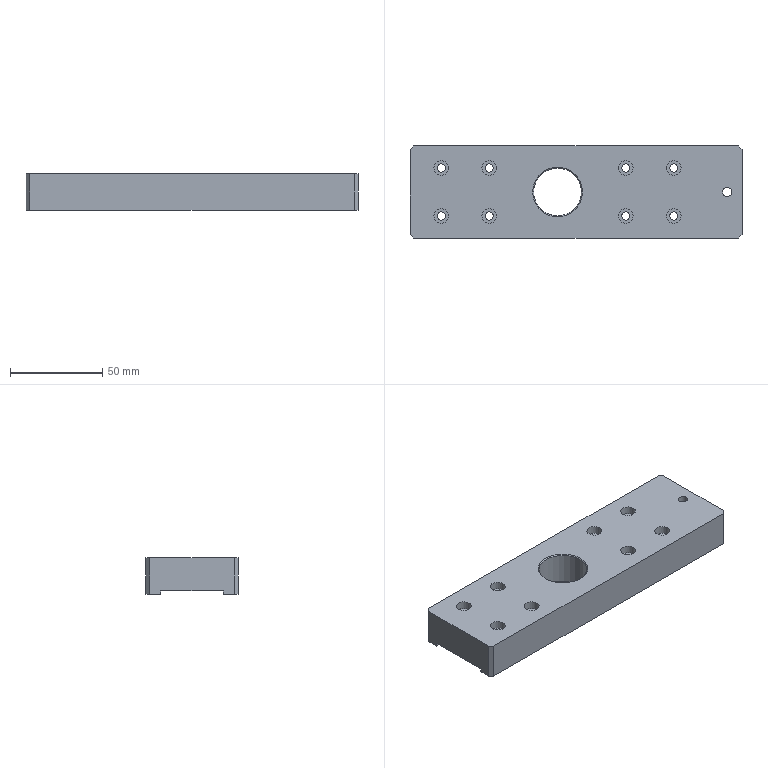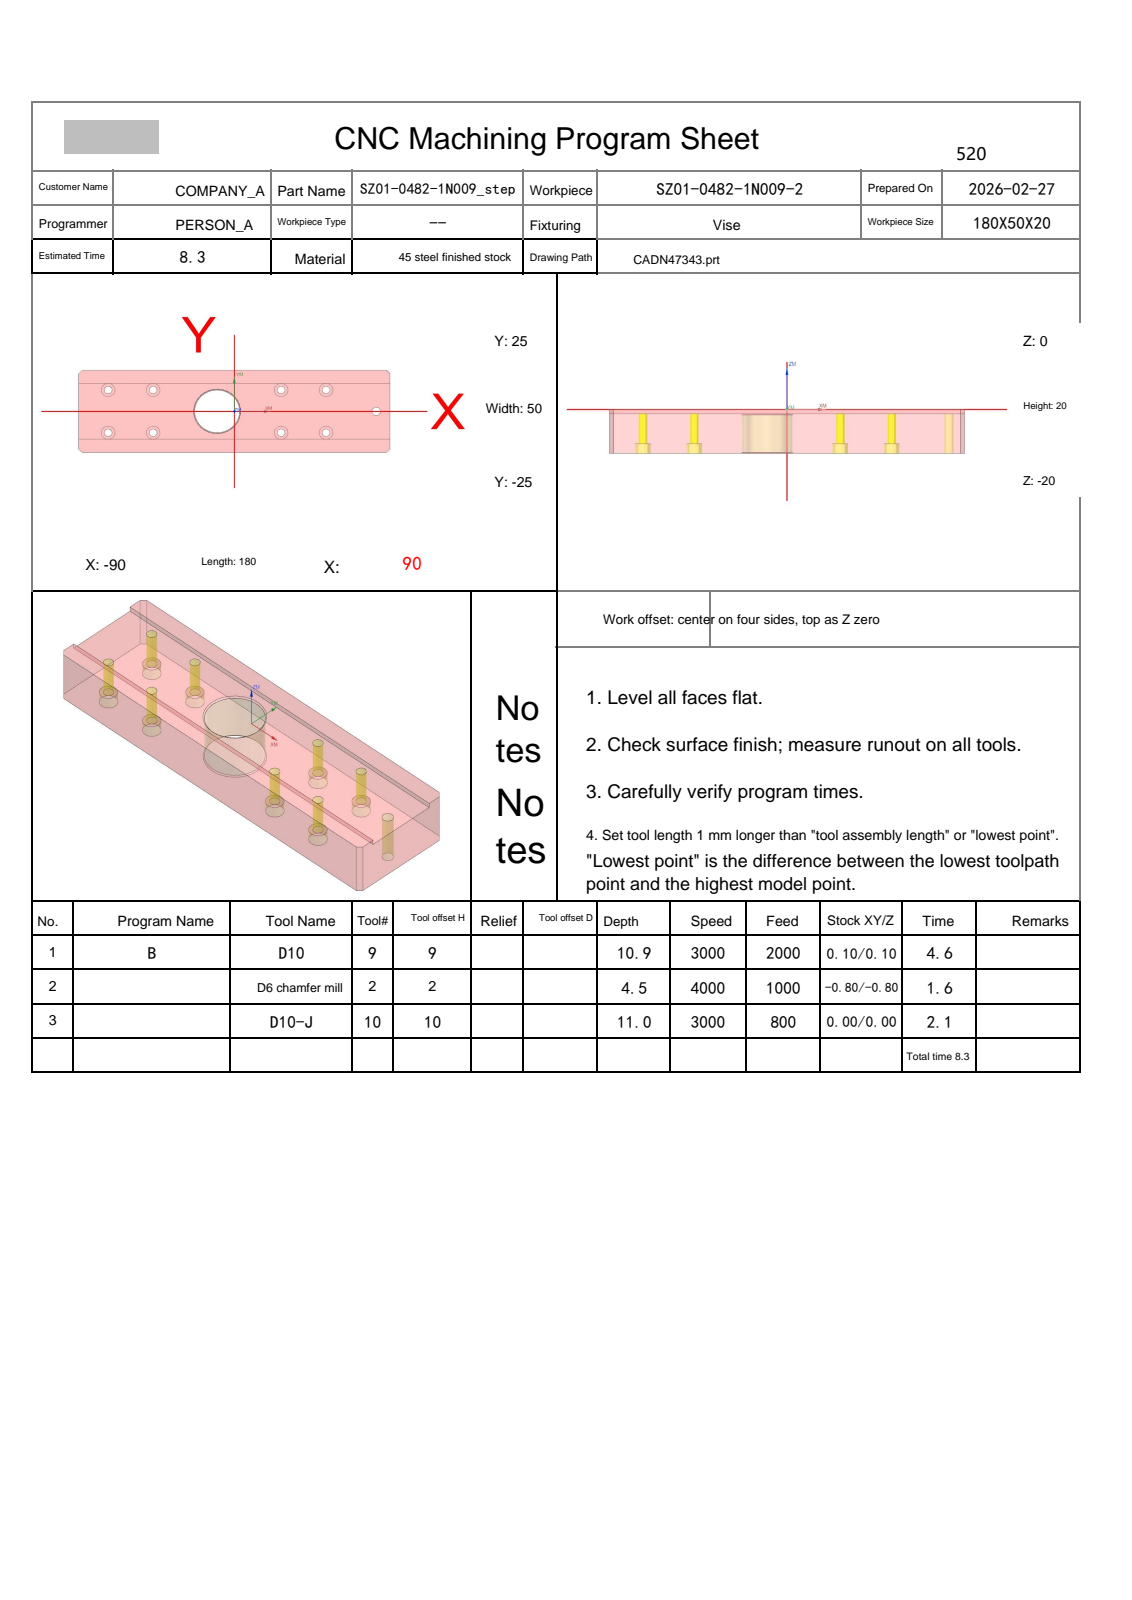NC program | NX | posted by the shop | part box 180 x 50 x 20 mm
Whole program:
%
O0001
(Machine time: 8.91 MIN)
(===Total Tool:3===)
(T9=D10     D=10.  R=0.   D-  H09 Z=-10.9 )
(T2=D6 chamfer mill   D=6.   R=0.   D-  H02 Z=-4.45 )
(T10=D10-J  D=10.  R=0.   D10 H10 Z=-11.  )
G80 G90 G17 G49 G40
G91 G28 Z0
M01
N1 T09 M06
(D10  D=10. R=0. H=09 ce=0.10 di=0.10)
T02
G00 G90 G54 X-85.242 Y-34.97 M03 S3000
G43 H09 Z30.
M08
Z-.5
G01 X-91.606 Y-28.606 F2000.
X-93.606 Y-26.606
X-99.97 Y-20.242
G00 Z-1.
G01 X-93.606 Y-26.606
X-91.606 Y-28.606
X-85.242 Y-34.97
G00 Z-1.5
G01 X-91.606 Y-28.606
X-93.606 Y-26.606
X-99.97 Y-20.242
G00 Z-2.
G01 X-93.606 Y-26.606
X-91.606 Y-28.606
X-85.242 Y-34.97
G00 Z-2.5
G01 X-91.606 Y-28.606
X-93.606 Y-26.606
X-99.97 Y-20.242
G00 Z-3.
G01 X-93.606 Y-26.606
X-91.606 Y-28.606
X-85.242 Y-34.97
G00 Z-3.5
G01 X-91.606 Y-28.606
X-93.606 Y-26.606
X-99.97 Y-20.242
G00 Z-4.
G01 X-93.606 Y-26.606
X-91.606 Y-28.606
X-85.242 Y-34.97
G00 Z-4.5
G01 X-91.606 Y-28.606
X-93.606 Y-26.606
X-99.97 Y-20.242
G00 Z-5.
G01 X-93.606 Y-26.606
X-91.606 Y-28.606
X-85.242 Y-34.97
G00 Z-5.5
G01 X-91.606 Y-28.606
X-93.606 Y-26.606
X-99.97 Y-20.242
G00 Z-6.
G01 X-93.606 Y-26.606
X-91.606 Y-28.606
X-85.242 Y-34.97
G00 Z-6.5
G01 X-91.606 Y-28.606
X-93.606 Y-26.606
X-99.97 Y-20.242
G00 Z-7.
G01 X-93.606 Y-26.606
X-91.606 Y-28.606
X-85.242 Y-34.97
G00 Z-7.5
G01 X-91.606 Y-28.606
X-93.606 Y-26.606
X-99.97 Y-20.242
G00 Z-8.
G01 X-93.606 Y-26.606
X-91.606 Y-28.606
X-85.242 Y-34.97
G00 Z-8.5
G01 X-91.606 Y-28.606
X-93.606 Y-26.606
X-99.97 Y-20.242
G00 Z-9.
G01 X-93.606 Y-26.606
X-91.606 Y-28.606
X-85.242 Y-34.97
G00 Z-9.5
G01 X-91.606 Y-28.606
X-93.606 Y-26.606
X-99.97 Y-20.242
G00 Z-10.
G01 X-93.606 Y-26.606
X-91.606 Y-28.606
X-85.242 Y-34.97
G00 Z-10.5
G01 X-91.606 Y-28.606
X-93.606 Y-26.606
X-99.97 Y-20.242
G00 Z-10.9
G01 X-93.606 Y-26.606
X-91.606 Y-28.606
X-85.242 Y-34.97
G00 Z30.
X-99.97 Y20.242
Z-.5
G01 X-93.606 Y26.606
X-91.606 Y28.606
X-85.242 Y34.97
G00 Z-1.
G01 X-91.606 Y28.606
X-93.606 Y26.606
X-99.97 Y20.242
G00 Z-1.5
G01 X-93.606 Y26.606
X-91.606 Y28.606
X-85.242 Y34.97
G00 Z-2.
G01 X-91.606 Y28.606
X-93.606 Y26.606
X-99.97 Y20.242
G00 Z-2.5
G01 X-93.606 Y26.606
X-91.606 Y28.606
X-85.242 Y34.97
G00 Z-3.
G01 X-91.606 Y28.606
X-93.606 Y26.606
X-99.97 Y20.242
G00 Z-3.5
G01 X-93.606 Y26.606
X-91.606 Y28.606
X-85.242 Y34.97
G00 Z-4.
G01 X-91.606 Y28.606
X-93.606 Y26.606
X-99.97 Y20.242
G00 Z-4.5
G01 X-93.606 Y26.606
X-91.606 Y28.606
X-85.242 Y34.97
G00 Z-5.
G01 X-91.606 Y28.606
X-93.606 Y26.606
X-99.97 Y20.242
G00 Z-5.5
G01 X-93.606 Y26.606
X-91.606 Y28.606
X-85.242 Y34.97
G00 Z-6.
G01 X-91.606 Y28.606
X-93.606 Y26.606
X-99.97 Y20.242
G00 Z-6.5
G01 X-93.606 Y26.606
X-91.606 Y28.606
X-85.242 Y34.97
G00 Z-7.
G01 X-91.606 Y28.606
X-93.606 Y26.606
X-99.97 Y20.242
G00 Z-7.5
G01 X-93.606 Y26.606
X-91.606 Y28.606
X-85.242 Y34.97
G00 Z-8.
G01 X-91.606 Y28.606
X-93.606 Y26.606
X-99.97 Y20.242
G00 Z-8.5
G01 X-93.606 Y26.606
X-91.606 Y28.606
X-85.242 Y34.97
G00 Z-9.
G01 X-91.606 Y28.606
X-93.606 Y26.606
X-99.97 Y20.242
G00 Z-9.5
G01 X-93.606 Y26.606
X-91.606 Y28.606
X-85.242 Y34.97
G00 Z-10.
G01 X-91.606 Y28.606
X-93.606 Y26.606
X-99.97 Y20.242
G00 Z-10.5
G01 X-93.606 Y26.606
X-91.606 Y28.606
X-85.242 Y34.97
G00 Z-10.9
G01 X-91.606 Y28.606
X-93.606 Y26.606
X-99.97 Y20.242
G00 Z30.
X85.242 Y34.97
Z-.5
G01 X91.606 Y28.606
X93.606 Y26.606
X99.97 Y20.242
G00 Z-1.
G01 X93.606 Y26.606
X91.606 Y28.606
X85.242 Y34.97
G00 Z-1.5
G01 X91.606 Y28.606
X93.606 Y26.606
X99.97 Y20.242
G00 Z-2.
G01 X93.606 Y26.606
X91.606 Y28.606
X85.242 Y34.97
G00 Z-2.5
G01 X91.606 Y28.606
X93.606 Y26.606
X99.97 Y20.242
G00 Z-3.
G01 X93.606 Y26.606
X91.606 Y28.606
X85.242 Y34.97
G00 Z-3.5
G01 X91.606 Y28.606
X93.606 Y26.606
X99.97 Y20.242
G00 Z-4.
G01 X93.606 Y26.606
X91.606 Y28.606
X85.242 Y34.97
G00 Z-4.5
G01 X91.606 Y28.606
X93.606 Y26.606
X99.97 Y20.242
G00 Z-5.
G01 X93.606 Y26.606
X91.606 Y28.606
X85.242 Y34.97
G00 Z-5.5
G01 X91.606 Y28.606
X93.606 Y26.606
X99.97 Y20.242
G00 Z-6.
G01 X93.606 Y26.606
X91.606 Y28.606
X85.242 Y34.97
G00 Z-6.5
G01 X91.606 Y28.606
X93.606 Y26.606
X99.97 Y20.242
G00 Z-7.
G01 X93.606 Y26.606
X91.606 Y28.606
X85.242 Y34.97
G00 Z-7.5
G01 X91.606 Y28.606
X93.606 Y26.606
X99.97 Y20.242
G00 Z-8.
G01 X93.606 Y26.606
X91.606 Y28.606
X85.242 Y34.97
G00 Z-8.5
G01 X91.606 Y28.606
X93.606 Y26.606
X99.97 Y20.242
G00 Z-9.
G01 X93.606 Y26.606
X91.606 Y28.606
X85.242 Y34.97
G00 Z-9.5
G01 X91.606 Y28.606
X93.606 Y26.606
X99.97 Y20.242
G00 Z-10.
G01 X93.606 Y26.606
X91.606 Y28.606
X85.242 Y34.97
G00 Z-10.5
G01 X91.606 Y28.606
X93.606 Y26.606
X99.97 Y20.242
G00 Z-10.9
G01 X93.606 Y26.606
X91.606 Y28.606
X85.242 Y34.97
G00 Z30.
X99.97 Y-20.242
Z-.5
G01 X93.606 Y-26.606
X91.606 Y-28.606
X85.242 Y-34.97
G00 Z-1.
G01 X91.606 Y-28.606
X93.606 Y-26.606
X99.97 Y-20.242
G00 Z-1.5
G01 X93.606 Y-26.606
X91.606 Y-28.606
X85.242 Y-34.97
G00 Z-2.
G01 X91.606 Y-28.606
X93.606 Y-26.606
X99.97 Y-20.242
G00 Z-2.5
G01 X93.606 Y-26.606
X91.606 Y-28.606
X85.242 Y-34.97
G00 Z-3.
G01 X91.606 Y-28.606
X93.606 Y-26.606
X99.97 Y-20.242
G00 Z-3.5
G01 X93.606 Y-26.606
X91.606 Y-28.606
X85.242 Y-34.97
G00 Z-4.
G01 X91.606 Y-28.606
X93.606 Y-26.606
X99.97 Y-20.242
G00 Z-4.5
G01 X93.606 Y-26.606
X91.606 Y-28.606
X85.242 Y-34.97
G00 Z-5.
G01 X91.606 Y-28.606
X93.606 Y-26.606
X99.97 Y-20.242
G00 Z-5.5
G01 X93.606 Y-26.606
X91.606 Y-28.606
X85.242 Y-34.97
G00 Z-6.
G01 X91.606 Y-28.606
X93.606 Y-26.606
X99.97 Y-20.242
G00 Z-6.5
G01 X93.606 Y-26.606
X91.606 Y-28.606
X85.242 Y-34.97
G00 Z-7.
G01 X91.606 Y-28.606
X93.606 Y-26.606
X99.97 Y-20.242
G00 Z-7.5
G01 X93.606 Y-26.606
X91.606 Y-28.606
X85.242 Y-34.97
G00 Z-8.
G01 X91.606 Y-28.606
X93.606 Y-26.606
X99.97 Y-20.242
G00 Z-8.5
G01 X93.606 Y-26.606
X91.606 Y-28.606
X85.242 Y-34.97
G00 Z-9.
G01 X91.606 Y-28.606
X93.606 Y-26.606
X99.97 Y-20.242
G00 Z-9.5
G01 X93.606 Y-26.606
X91.606 Y-28.606
X85.242 Y-34.97
G00 Z-10.
G01 X91.606 Y-28.606
X93.606 Y-26.606
X99.97 Y-20.242
G00 Z-10.5
G01 X93.606 Y-26.606
X91.606 Y-28.606
X85.242 Y-34.97
G00 Z-10.9
G01 X91.606 Y-28.606
X93.606 Y-26.606
X99.97 Y-20.242
G00 Z30.
G00 G90 X98. Y0.0 M03 S3000
Z10.1
Z1.3
G01 Z-.2 F2000.
X94.9
Y-11.8
X-94.9
Y11.8
X94.9
Y3.035
G02 X94.455 Y2.203 I-1. J0.0
G01 X87.845 Y-2.204
G03 X87.4 Y-3.034 I.555 J-.832
G01 Y-3.303
G02 X86.403 Y-4.3 I-1. J.003
G01 X-86.403
G02 X-87.4 Y-3.303 I.003 J1.
G01 Y3.303
G02 X-86.403 Y4.3 I1. J-.003
G01 X86.403
G02 X87.4 Y3.303 I-.003 J-1.
G01 Y0.0
Y-.5
X98.
Z1.3
G00 Y0.0
Z1.1
G01 Z-.4
X94.9
Y-11.8
X-94.9
Y11.8
X94.9
Y3.035
G02 X94.455 Y2.203 I-1. J0.0
G01 X87.845 Y-2.204
G03 X87.4 Y-3.034 I.555 J-.832
G01 Y-3.303
G02 X86.403 Y-4.3 I-1. J.003
G01 X-86.403
G02 X-87.4 Y-3.303 I.003 J1.
G01 Y3.303
G02 X-86.403 Y4.3 I1. J-.003
G01 X86.403
G02 X87.4 Y3.303 I-.003 J-1.
G01 Y0.0
Y-.5
X98.
Z1.1
G00 Y0.0
Z.9
G01 Z-.6
X94.9
Y-11.8
X-94.9
Y11.8
X94.9
Y3.035
G02 X94.455 Y2.203 I-1. J0.0
G01 X87.845 Y-2.204
G03 X87.4 Y-3.034 I.555 J-.832
G01 Y-3.303
G02 X86.403 Y-4.3 I-1. J.003
G01 X-86.403
G02 X-87.4 Y-3.303 I.003 J1.
G01 Y3.303
G02 X-86.403 Y4.3 I1. J-.003
G01 X86.403
G02 X87.4 Y3.303 I-.003 J-1.
G01 Y0.0
Y-.5
X98.
Z.9
G00 Y0.0
Z.7
G01 Z-.8
X94.9
Y-11.8
X-94.9
Y11.8
X94.9
Y3.035
G02 X94.455 Y2.203 I-1. J0.0
G01 X87.845 Y-2.204
G03 X87.4 Y-3.034 I.555 J-.832
G01 Y-3.303
G02 X86.403 Y-4.3 I-1. J.003
G01 X-86.403
G02 X-87.4 Y-3.303 I.003 J1.
G01 Y3.303
G02 X-86.403 Y4.3 I1. J-.003
G01 X86.403
G02 X87.4 Y3.303 I-.003 J-1.
G01 Y0.0
Y-.5
X98.
Z.7
G00 Y0.0
Z.5
G01 Z-1.
X94.9
Y-11.8
X-94.9
Y11.8
X94.9
Y3.035
G02 X94.455 Y2.203 I-1. J0.0
G01 X87.845 Y-2.204
G03 X87.4 Y-3.034 I.555 J-.832
G01 Y-3.303
G02 X86.403 Y-4.3 I-1. J.003
G01 X-86.403
G02 X-87.4 Y-3.303 I.003 J1.
G01 Y3.303
G02 X-86.403 Y4.3 I1. J-.003
G01 X86.403
G02 X87.4 Y3.303 I-.003 J-1.
G01 Y0.0
Y-.5
X98.
Z.5
G00 Y0.0
Z.3
G01 Z-1.2
X94.9
Y-11.8
X-94.9
Y11.8
X94.9
Y3.035
G02 X94.455 Y2.203 I-1. J0.0
G01 X87.845 Y-2.204
G03 X87.4 Y-3.034 I.555 J-.832
G01 Y-3.303
G02 X86.403 Y-4.3 I-1. J.003
G01 X-86.403
G02 X-87.4 Y-3.303 I.003 J1.
G01 Y3.303
G02 X-86.403 Y4.3 I1. J-.003
G01 X86.403
G02 X87.4 Y3.303 I-.003 J-1.
G01 Y0.0
Y-.5
X98.
Z.3
G00 Y0.0
Z.1
G01 Z-1.4
X94.9
Y-11.8
X-94.9
Y11.8
X94.9
Y3.035
G02 X94.455 Y2.203 I-1. J0.0
G01 X87.845 Y-2.204
G03 X87.4 Y-3.034 I.555 J-.832
G01 Y-3.303
G02 X86.403 Y-4.3 I-1. J.003
G01 X-86.403
G02 X-87.4 Y-3.303 I.003 J1.
G01 Y3.303
G02 X-86.403 Y4.3 I1. J-.003
G01 X86.403
G02 X87.4 Y3.303 I-.003 J-1.
G01 Y0.0
Y-.5
X98.
Z.1
G00 Y0.0
Z-.1
G01 Z-1.6
X94.9
Y-11.8
X-94.9
Y11.8
X94.9
Y3.035
G02 X94.455 Y2.203 I-1. J0.0
G01 X87.845 Y-2.204
G03 X87.4 Y-3.034 I.555 J-.832
G01 Y-3.303
G02 X86.403 Y-4.3 I-1. J.003
G01 X-86.403
G02 X-87.4 Y-3.303 I.003 J1.
G01 Y3.303
G02 X-86.403 Y4.3 I1. J-.003
G01 X86.403
G02 X87.4 Y3.303 I-.003 J-1.
G01 Y0.0
Y-.5
X98.
Z-.1
G00 Y0.0
Z-.3
G01 Z-1.8
X94.9
Y-11.8
X-94.9
Y11.8
X94.9
Y3.035
G02 X94.455 Y2.203 I-1. J0.0
G01 X87.845 Y-2.204
G03 X87.4 Y-3.034 I.555 J-.832
G01 Y-3.303
G02 X86.403 Y-4.3 I-1. J.003
G01 X-86.403
G02 X-87.4 Y-3.303 I.003 J1.
G01 Y3.303
G02 X-86.403 Y4.3 I1. J-.003
G01 X86.403
G02 X87.4 Y3.303 I-.003 J-1.
G01 Y0.0
Y-.5
X98.
Z-.3
G00 Z10.1
G91 G28 Z0.0
M05
M09
G91 G28 Z0.0
M01
N2 T02 M06
(D6 chamfer mill  D=6. R=0. H=02 ce=0.00 di=0.10)
T10
G00 G90 G54 X27. Y-13. M03 S2000
G43 H02 Z30.
M08
G98 G81 X27. Y-13. Z-4.45 R1.1 F100.
X53.
Y13.
X27.
X-47.
Y-13.
X-73.
Y13.
G80
G00 Z30.
G00 G90 X81.907 Y.694 M03 S4000
Z30.
Z-3.
G01 Z-3.5 F300.
X81.8 Y1.5
G03 X80.3 Y0.0 I0.0 J-1.5
X82. Y-1.7 I1.7 J0.0
X83.7 Y0.0 I0.0 J1.7
X82. Y1.7 I-1.7 J0.0
X80.3 Y0.0 I0.0 J-1.7
X81.8 Y-1.5 I1.5 J0.0
G01 X81.907 Y-.694
Z-3.
G00 Z30.
G00 G90 X-8.8 Y11.035 M03 S3500
Z30.
Z-1.7
G01 Z-3.2 F1000.
Y11.1
G03 X-10. Y12.3 I-1.2 J0.0
X-22.3 Y0.0 I0.0 J-12.3
X-10. Y-12.3 I12.3 J0.0
X2.3 Y0.0 I0.0 J12.3
X-10. Y12.3 I-12.3 J0.0
X-10.4 Y12.293 I0.0 J-12.3
X-11.561 Y11.094 I.039 J-1.199
G01 X-11.56 Y11.055
X-11.558 Y10.99
Z-1.7
G00 Z30.
G00 G90 X.386 Y15.673 M03 S3500
Z30.
Z.172
G01 Z-1.2 F1000.
G03 X.1 Y15.873 I-1.286 J-1.532
G01 X.054 Y15.903
X0.0 Y15.9
X-90.
G02 X-91. Y16.9 I0.0 J1.
G01 Y23.
X-90.966 Y23.259
X-90.866 Y23.5
X-90.707 Y23.707
X-88.707 Y25.707
X-88.5 Y25.866
X-88.259 Y25.966
X-88. Y26.
X88.
X88.259 Y25.966
X88.5 Y25.866
X88.707 Y25.707
X90.707 Y23.707
X90.866 Y23.5
X90.966 Y23.259
X91. Y23.
Y16.9
G02 X90. Y15.9 I-1. J0.0
G01 X0.0
X-.054 Y15.903
X-.1 Y15.873
G03 X-.386 Y15.673 I1. J-1.732
G01 Z.172
G00 Z10.
Y-15.673
Z.172
G01 Z-1.2
G03 X-.1 Y-15.873 I1.286 J1.532
G01 X-.054 Y-15.903
X0.0 Y-15.9
X90.
G02 X91. Y-16.9 I0.0 J-1.
G01 Y-23.
X90.966 Y-23.259
X90.866 Y-23.5
X90.707 Y-23.707
X88.707 Y-25.707
X88.5 Y-25.866
X88.259 Y-25.966
X88. Y-26.
X-88.
X-88.259 Y-25.966
X-88.5 Y-25.866
X-88.707 Y-25.707
X-90.707 Y-23.707
X-90.866 Y-23.5
X-90.966 Y-23.259
X-91. Y-23.
Y-16.9
G02 X-90. Y-15.9 I1. J0.0
G01 X0.0
X.054 Y-15.903
X.1 Y-15.873
G03 X.386 Y-15.673 I-1. J1.732
G01 Z.172
G00 Z10.
X-91.136 Y-14.128
Z-1.597
G01 Z-3.1
G03 X-91.016 Y-13.956 I-.919 J.771
G01 X-90.994 Y-13.93
X-91. Y-13.896
Y13.896
X-90.994 Y13.93
X-91.016 Y13.956
G03 X-91.136 Y14.128 I-1.039 J-.6
G01 Z-1.597
G00 Z10.
X91.136
Z-1.597
G01 Z-3.1
G03 X91.016 Y13.956 I.919 J-.771
G01 X90.994 Y13.93
X91. Y13.896
Y-13.896
X90.994 Y-13.93
X91.016 Y-13.956
G03 X91.136 Y-14.128 I1.039 J.6
G01 Z-1.597
G00 Z10.
X80.685 Y.407
Z-1.616
G01 Z-3.1
G03 X80.516 Y.102 I1.658 J-1.118
G01 X80.491 Y.054
X80.5 Y0.0
G03 X82. Y-1.5 I1.5 J0.0
X83.5 Y0.0 I0.0 J1.5
X82. Y1.5 I-1.5 J0.0
X80.5 Y0.0 I0.0 J-1.5
G01 X80.491 Y-.054
X80.516 Y-.102
G03 X80.685 Y-.407 I1.827 J.813
G01 Z-1.616
G00 Z10.
X53.656 Y-13.89
Z-1.611
G01 Z-3.1
G03 X53.948 Y-13.774 I-.516 J1.724
G01 X53.993 Y-13.756
X54.017 Y-13.713
X54.117 Y-13.561
G03 X54.25 Y-13. I-1.117 J.561
X53. Y-11.75 I-1.25 J0.0
X51.75 Y-13. I0.0 J-1.25
X51.989 Y-13.735 I1.25 J0.0
G01 X52.004 Y-13.771
X52.04 Y-13.786
G03 X52.261 Y-13.889 I.7 J1.212
G01 Z-1.587
G00 Z10.
Y13.889
Z-1.587
G01 Z-3.1
G03 X52.04 Y13.786 I.479 J-1.316
G01 X52.004 Y13.771
X51.989 Y13.735
G03 X51.75 Y13. I1.011 J-.735
X53. Y11.75 I1.25 J0.0
X54.25 Y13. I0.0 J1.25
X54.117 Y13.561 I-1.25 J0.0
G01 X54.017 Y13.713
X53.993 Y13.756
X53.948 Y13.774
G03 X53.656 Y13.89 I-.808 J-1.609
G01 Z-1.611
G00 Z10.
X26.261 Y13.889
Z-1.587
G01 Z-3.1
G03 X26.04 Y13.786 I.479 J-1.316
G01 X26.004 Y13.771
X25.989 Y13.735
G03 X25.75 Y13. I1.011 J-.735
X27. Y11.75 I1.25 J0.0
X28.25 Y13. I0.0 J1.25
X28.117 Y13.561 I-1.25 J0.0
G01 X28.017 Y13.713
X27.993 Y13.756
X27.948 Y13.774
G03 X27.656 Y13.89 I-.808 J-1.609
G01 Z-1.611
G00 Z10.
Y-13.89
Z-1.611
G01 Z-3.1
G03 X27.948 Y-13.774 I-.516 J1.724
G01 X27.993 Y-13.756
X28.017 Y-13.713
X28.117 Y-13.561
G03 X28.25 Y-13. I-1.117 J.561
X27. Y-11.75 I-1.25 J0.0
X25.75 Y-13. I0.0 J-1.25
X25.989 Y-13.735 I1.25 J0.0
G01 X26.004 Y-13.771
X26.04 Y-13.786
G03 X26.261 Y-13.889 I.7 J1.212
G01 Z-1.587
G00 Z10.
X-46.344 Y-13.89
Z-1.611
G01 Z-3.1
G03 X-46.052 Y-13.774 I-.516 J1.724
G01 X-46.007 Y-13.756
X-45.983 Y-13.713
X-45.883 Y-13.561
G03 X-45.75 Y-13. I-1.117 J.561
X-47. Y-11.75 I-1.25 J0.0
X-48.25 Y-13. I0.0 J-1.25
X-48.011 Y-13.735 I1.25 J0.0
G01 X-47.996 Y-13.771
X-47.96 Y-13.786
G03 X-47.739 Y-13.889 I.7 J1.212
G01 Z-1.587
G00 Z10.
X-72.344 Y-13.89
Z-1.611
G01 Z-3.1
G03 X-72.052 Y-13.774 I-.516 J1.724
G01 X-72.007 Y-13.756
X-71.983 Y-13.713
X-71.883 Y-13.561
G03 X-71.75 Y-13. I-1.117 J.561
X-73. Y-11.75 I-1.25 J0.0
X-74.25 Y-13. I0.0 J-1.25
X-74.011 Y-13.735 I1.25 J0.0
G01 X-73.996 Y-13.771
X-73.96 Y-13.786
G03 X-73.739 Y-13.889 I.7 J1.212
G01 Z-1.587
G00 Z10.
Y13.889
Z-1.587
G01 Z-3.1
G03 X-73.96 Y13.786 I.479 J-1.316
G01 X-73.996 Y13.771
X-74.011 Y13.735
G03 X-74.25 Y13. I1.011 J-.735
X-73. Y11.75 I1.25 J0.0
X-71.75 Y13. I0.0 J1.25
X-71.883 Y13.561 I-1.25 J0.0
G01 X-71.983 Y13.713
X-72.007 Y13.756
X-72.052 Y13.774
G03 X-72.344 Y13.89 I-.808 J-1.609
G01 Z-1.611
G00 Z10.
X-47.739 Y13.889
Z-1.587
G01 Z-3.1
G03 X-47.96 Y13.786 I.479 J-1.316
G01 X-47.996 Y13.771
X-48.011 Y13.735
X-48.142 Y13.508
X-48.223 Y13.26
X-48.25 Y13.
G03 X-47. Y11.75 I1.25 J0.0
X-45.75 Y13. I0.0 J1.25
X-45.883 Y13.561 I-1.25 J0.0
G01 X-45.983 Y13.713
X-46.007 Y13.756
X-46.052 Y13.774
G03 X-46.344 Y13.89 I-.808 J-1.609
G01 Z-1.611
G00 Z30.
G91 G28 Z0.0
M05
M09
G91 G28 Z0.0
M01
N3 T10 M06
(D10-J  D=10. R=0. H=10 ce=0.40 di=0.00)
T09
G00 G90 G54 X-97. Y-2. M03 S3000
G43 H10 Z10.4
M08
Z-.4
G01 Z-1.9 F800.
X-93.
G03 X-91. Y0.0 I0.0 J2.
G01 Y10.504
G02 X-90.004 Y11.5 I1. J-.004
G01 X90.004
G02 X91. Y10.504 I-.004 J-1.
G01 Y-10.504
G02 X90.004 Y-11.5 I-1. J.004
G01 X-90.004
G02 X-91. Y-10.504 I.004 J1.
G01 Y1.934
G02 X-90.515 Y2.791 I1. J0.0
G01 X-86.382 Y5.275
G03 X-85.949 Y5.815 I-.516 J.857
G02 X-85.004 Y6.5 I.949 J-.315
G01 X85.004
G02 X86. Y5.504 I-.004 J-1.
G01 Y-5.504
G02 X85.004 Y-6.5 I-1. J.004
G01 X-85.004
G02 X-86. Y-5.504 I.004 J1.
G01 Y1.588
G02 X-85.2 Y2.387 I.8 J0.0
G01 X-85.096 Y2.381
X-78.492 Y1.508
X-78.362 Y1.5
X80.005
G02 X81. Y.505 I-.004 J-1.
G01 Y-.505
G02 X80.005 Y-1.5 I-1. J.004
G01 X-80.005
G02 X-81. Y-.505 I.005 J1.
G01 Y.505
G02 X-80.8 Y1.1 I1. J-.005
X-80.005 Y1.5 I.8 J-.6
G01 X-79.927
G03 X-77.927 Y3.5 I0.0 J2.
G01 Z-.4
G00 Z10.4
G00 G90 X97. Y9.701 M03 S3000
Z10.1
Z-.9
G01 Z-1.9 F800.
G41 D10
Y9.901
G03 X95. Y11.9 I-2. J-.001
G01 X-95.
G03 X-97. Y9.901 I0.0 J-2.
G01 G40 Y9.701
Z-.9
G00 Y-9.701
G01 Z-1.9
G41 D10
Y-9.901
G03 X-95. Y-11.9 I2. J.001
G01 X95.
G03 X97. Y-9.901 I0.0 J2.
G01 G40 Y-9.701
Z-.9
G00 Z10.1
G00 G90 X-87.293 Y-32.778 M03 S3000
Z30.
Z-10.
G01 Z-11. F800.
X-91.536 Y-28.536
X-93.536 Y-26.536
X-97.778 Y-22.293
Z-10.
G00 Z30.
Y22.293
Z-10.
G01 Z-11.
X-93.536 Y26.536
X-91.536 Y28.536
X-87.293 Y32.778
Z-10.
G00 Z30.
X87.293
Z-10.
G01 Z-11.
X91.536 Y28.536
X93.536 Y26.536
X97.778 Y22.293
Z-10.
G00 Z30.
Y-22.293
Z-10.
G01 Z-11.
X93.536 Y-26.536
X91.536 Y-28.536
X87.293 Y-32.778
Z-10.
G00 Z30.
M05
M09
G91 G28 Z0.0
G91 G28 Y0.0
M30
%